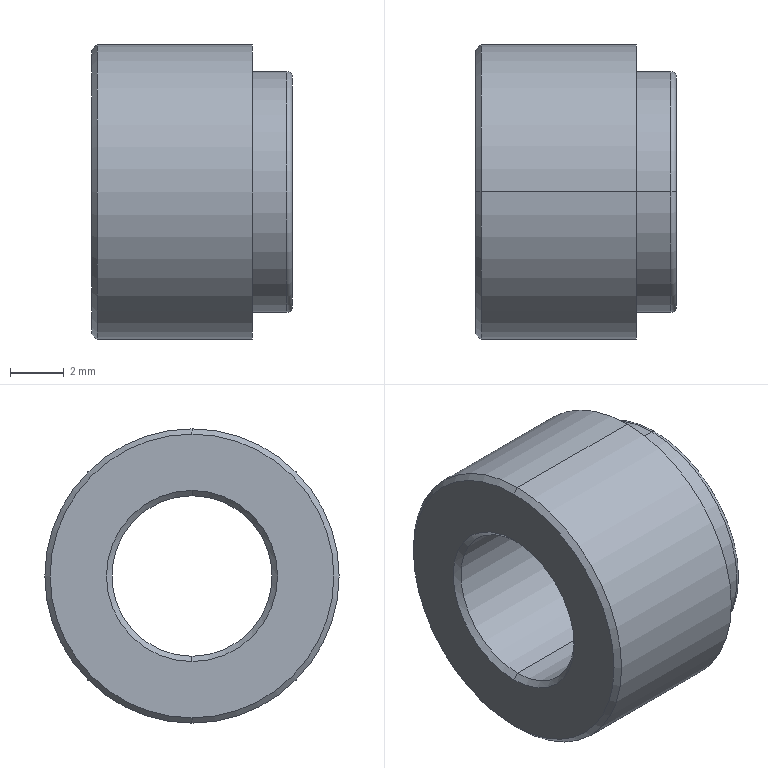Part | SolidWorks | features Chamfer 1, Extrusion 1, Fillet 1, ICE 1 | 2 solids | 20 faces | box 7.5 x 11 x 11 mm | volume 452.095 mm3 | cylinder 8 | cone 4 | plane 4 | torus 4 | commonest cylinder face diameters 6 x4 9 x2 11 x2
STEP:
#1=CARTESIAN_POINT('',(0.,0.,5.3));
#2=VERTEX_POINT('',#1);
#3=CARTESIAN_POINT('',(0.,0.,-5.3));
#4=VERTEX_POINT('',#3);
#5=CARTESIAN_POINT('',(0.,0.,0.));
#6=DIRECTION('',(-1.,0.,0.));
#7=DIRECTION('',(0.,0.,-1.));
#8=AXIS2_PLACEMENT_3D('',#5,#6,#7);
#9=CIRCLE('',#8,5.3);
#10=EDGE_CURVE('',#2,#4,#9,.T.);
#11=ORIENTED_EDGE('',*,*,#10,.F.);
#12=CARTESIAN_POINT('',(0.2,0.,5.5));
#13=VERTEX_POINT('',#12);
#14=CARTESIAN_POINT('',(0.2,0.,5.5));
#15=DIRECTION('',(0.7071,0.,0.7071));
#16=VECTOR('',#15,1000.);
#17=LINE('',#14,#16);
#18=EDGE_CURVE('',#2,#13,#17,.T.);
#19=ORIENTED_EDGE('',*,*,#18,.T.);
#20=CARTESIAN_POINT('',(0.2,0.,-5.5));
#21=VERTEX_POINT('',#20);
#22=CARTESIAN_POINT('',(0.2,0.,0.));
#23=DIRECTION('',(1.,0.,0.));
#24=DIRECTION('',(0.,0.,-1.));
#25=AXIS2_PLACEMENT_3D('',#22,#23,#24);
#26=CIRCLE('',#25,5.5);
#27=EDGE_CURVE('',#21,#13,#26,.T.);
#28=ORIENTED_EDGE('',*,*,#27,.F.);
#29=CARTESIAN_POINT('',(0.2,0.,-5.5));
#30=DIRECTION('',(0.7071,0.,-0.7071));
#31=VECTOR('',#30,1000.);
#32=LINE('',#29,#31);
#33=EDGE_CURVE('',#4,#21,#32,.T.);
#34=ORIENTED_EDGE('',*,*,#33,.F.);
#35=EDGE_LOOP('',(#11,#19,#28,#34));
#36=FACE_OUTER_BOUND('',#35,.T.);
#37=CARTESIAN_POINT('',(0.2,0.,0.));
#38=DIRECTION('',(1.,0.,0.));
#39=DIRECTION('',(0.,0.,-1.));
#40=AXIS2_PLACEMENT_3D('',#37,#38,#39);
#41=CONICAL_SURFACE('',#40,5.5,0.7854);
#42=ADVANCED_FACE('',(#36),#41,.T.);
#43=CARTESIAN_POINT('',(0.2,0.,-3.));
#44=VERTEX_POINT('',#43);
#45=CARTESIAN_POINT('',(0.2,0.,3.));
#46=VERTEX_POINT('',#45);
#47=CARTESIAN_POINT('',(0.2,0.,0.));
#48=DIRECTION('',(-1.,0.,0.));
#49=DIRECTION('',(0.,0.,-1.));
#50=AXIS2_PLACEMENT_3D('',#47,#48,#49);
#51=CIRCLE('',#50,3.);
#52=EDGE_CURVE('',#44,#46,#51,.T.);
#53=ORIENTED_EDGE('',*,*,#52,.F.);
#54=CARTESIAN_POINT('',(0.,0.,-3.2));
#55=VERTEX_POINT('',#54);
#56=CARTESIAN_POINT('',(0.,0.,-3.2));
#57=DIRECTION('',(-0.7071,0.,-0.7071));
#58=VECTOR('',#57,1000.);
#59=LINE('',#56,#58);
#60=EDGE_CURVE('',#44,#55,#59,.T.);
#61=ORIENTED_EDGE('',*,*,#60,.T.);
#62=CARTESIAN_POINT('',(0.,0.,3.2));
#63=VERTEX_POINT('',#62);
#64=CARTESIAN_POINT('',(0.,0.,0.));
#65=DIRECTION('',(1.,0.,0.));
#66=DIRECTION('',(0.,0.,-1.));
#67=AXIS2_PLACEMENT_3D('',#64,#65,#66);
#68=CIRCLE('',#67,3.2);
#69=EDGE_CURVE('',#63,#55,#68,.T.);
#70=ORIENTED_EDGE('',*,*,#69,.F.);
#71=CARTESIAN_POINT('',(0.,0.,3.2));
#72=DIRECTION('',(-0.7071,0.,0.7071));
#73=VECTOR('',#72,1000.);
#74=LINE('',#71,#73);
#75=EDGE_CURVE('',#46,#63,#74,.T.);
#76=ORIENTED_EDGE('',*,*,#75,.F.);
#77=EDGE_LOOP('',(#53,#61,#70,#76));
#78=FACE_OUTER_BOUND('',#77,.T.);
#79=CARTESIAN_POINT('',(0.,0.,0.));
#80=DIRECTION('',(-1.,0.,0.));
#81=DIRECTION('',(0.,0.,1.));
#82=AXIS2_PLACEMENT_3D('',#79,#80,#81);
#83=CONICAL_SURFACE('',#82,3.2,0.7854);
#84=ADVANCED_FACE('',(#78),#83,.F.);
#85=CARTESIAN_POINT('',(6.,0.,3.));
#86=VERTEX_POINT('',#85);
#87=CARTESIAN_POINT('',(6.,0.,-3.));
#88=VERTEX_POINT('',#87);
#89=CARTESIAN_POINT('',(6.,0.,0.));
#90=DIRECTION('',(1.,0.,0.));
#91=DIRECTION('',(0.,0.,-1.));
#92=AXIS2_PLACEMENT_3D('',#89,#90,#91);
#93=CIRCLE('',#92,3.);
#94=EDGE_CURVE('',#86,#88,#93,.T.);
#95=ORIENTED_EDGE('',*,*,#94,.T.);
#96=CARTESIAN_POINT('',(6.,0.,-3.));
#97=DIRECTION('',(-1.,0.,0.));
#98=VECTOR('',#97,1000.);
#99=LINE('',#96,#98);
#100=EDGE_CURVE('',#88,#44,#99,.T.);
#101=ORIENTED_EDGE('',*,*,#100,.T.);
#102=ORIENTED_EDGE('',*,*,#52,.T.);
#103=CARTESIAN_POINT('',(6.,0.,3.));
#104=DIRECTION('',(-1.,0.,0.));
#105=VECTOR('',#104,1000.);
#106=LINE('',#103,#105);
#107=EDGE_CURVE('',#86,#46,#106,.T.);
#108=ORIENTED_EDGE('',*,*,#107,.F.);
#109=EDGE_LOOP('',(#95,#101,#102,#108));
#110=FACE_OUTER_BOUND('',#109,.T.);
#111=CARTESIAN_POINT('',(6.,0.,0.));
#112=DIRECTION('',(-1.,0.,0.));
#113=DIRECTION('',(0.,0.,1.));
#114=AXIS2_PLACEMENT_3D('',#111,#112,#113);
#115=CYLINDRICAL_SURFACE('',#114,3.);
#116=ADVANCED_FACE('',(#110),#115,.F.);
#117=CARTESIAN_POINT('',(6.,0.,-5.5));
#118=VERTEX_POINT('',#117);
#119=CARTESIAN_POINT('',(6.,0.,5.5));
#120=VERTEX_POINT('',#119);
#121=CARTESIAN_POINT('',(6.,0.,0.));
#122=DIRECTION('',(1.,0.,0.));
#123=DIRECTION('',(0.,0.,-1.));
#124=AXIS2_PLACEMENT_3D('',#121,#122,#123);
#125=CIRCLE('',#124,5.5);
#126=EDGE_CURVE('',#118,#120,#125,.T.);
#127=ORIENTED_EDGE('',*,*,#126,.F.);
#128=CARTESIAN_POINT('',(6.,0.,-5.5));
#129=DIRECTION('',(-1.,0.,0.));
#130=VECTOR('',#129,1000.);
#131=LINE('',#128,#130);
#132=EDGE_CURVE('',#118,#21,#131,.T.);
#133=ORIENTED_EDGE('',*,*,#132,.T.);
#134=ORIENTED_EDGE('',*,*,#27,.T.);
#135=CARTESIAN_POINT('',(6.,0.,5.5));
#136=DIRECTION('',(-1.,0.,0.));
#137=VECTOR('',#136,1000.);
#138=LINE('',#135,#137);
#139=EDGE_CURVE('',#120,#13,#138,.T.);
#140=ORIENTED_EDGE('',*,*,#139,.F.);
#141=EDGE_LOOP('',(#127,#133,#134,#140));
#142=FACE_OUTER_BOUND('',#141,.T.);
#143=CARTESIAN_POINT('',(6.,0.,0.));
#144=DIRECTION('',(-1.,0.,0.));
#145=DIRECTION('',(0.,0.,1.));
#146=AXIS2_PLACEMENT_3D('',#143,#144,#145);
#147=CYLINDRICAL_SURFACE('',#146,5.5);
#148=ADVANCED_FACE('',(#142),#147,.T.);
#149=CARTESIAN_POINT('',(6.,0.,0.));
#150=DIRECTION('',(1.,0.,0.));
#151=DIRECTION('',(0.,0.,-1.));
#152=AXIS2_PLACEMENT_3D('',#149,#150,#151);
#153=CIRCLE('',#152,5.5);
#154=EDGE_CURVE('',#120,#118,#153,.T.);
#155=ORIENTED_EDGE('',*,*,#154,.T.);
#156=ORIENTED_EDGE('',*,*,#126,.T.);
#157=EDGE_LOOP('',(#155,#156));
#158=FACE_OUTER_BOUND('',#157,.T.);
#159=ORIENTED_EDGE('',*,*,#94,.F.);
#160=CARTESIAN_POINT('',(6.,0.,0.));
#161=DIRECTION('',(1.,0.,0.));
#162=DIRECTION('',(0.,0.,-1.));
#163=AXIS2_PLACEMENT_3D('',#160,#161,#162);
#164=CIRCLE('',#163,3.);
#165=EDGE_CURVE('',#88,#86,#164,.T.);
#166=ORIENTED_EDGE('',*,*,#165,.F.);
#167=EDGE_LOOP('',(#159,#166));
#168=FACE_BOUND('',#167,.T.);
#169=CARTESIAN_POINT('',(6.,0.,0.));
#170=DIRECTION('',(1.,0.,0.));
#171=DIRECTION('',(0.,0.,-1.));
#172=AXIS2_PLACEMENT_3D('',#169,#170,#171);
#173=PLANE('',#172);
#174=ADVANCED_FACE('',(#158,#168),#173,.T.);
#175=ORIENTED_EDGE('',*,*,#69,.T.);
#176=CARTESIAN_POINT('',(0.,0.,0.));
#177=DIRECTION('',(1.,0.,0.));
#178=DIRECTION('',(0.,0.,-1.));
#179=AXIS2_PLACEMENT_3D('',#176,#177,#178);
#180=CIRCLE('',#179,3.2);
#181=EDGE_CURVE('',#55,#63,#180,.T.);
#182=ORIENTED_EDGE('',*,*,#181,.T.);
#183=EDGE_LOOP('',(#175,#182));
#184=FACE_BOUND('',#183,.T.);
#185=CARTESIAN_POINT('',(0.,0.,0.));
#186=DIRECTION('',(-1.,0.,0.));
#187=DIRECTION('',(0.,0.,-1.));
#188=AXIS2_PLACEMENT_3D('',#185,#186,#187);
#189=CIRCLE('',#188,5.3);
#190=EDGE_CURVE('',#4,#2,#189,.T.);
#191=ORIENTED_EDGE('',*,*,#190,.T.);
#192=ORIENTED_EDGE('',*,*,#10,.T.);
#193=EDGE_LOOP('',(#191,#192));
#194=FACE_OUTER_BOUND('',#193,.T.);
#195=CARTESIAN_POINT('',(0.,0.,0.));
#196=DIRECTION('',(1.,0.,0.));
#197=DIRECTION('',(0.,0.,-1.));
#198=AXIS2_PLACEMENT_3D('',#195,#196,#197);
#199=PLANE('',#198);
#200=ADVANCED_FACE('',(#184,#194),#199,.F.);
#201=ORIENTED_EDGE('',*,*,#132,.F.);
#202=ORIENTED_EDGE('',*,*,#154,.F.);
#203=ORIENTED_EDGE('',*,*,#139,.T.);
#204=CARTESIAN_POINT('',(0.2,0.,0.));
#205=DIRECTION('',(1.,0.,0.));
#206=DIRECTION('',(0.,0.,-1.));
#207=AXIS2_PLACEMENT_3D('',#204,#205,#206);
#208=CIRCLE('',#207,5.5);
#209=EDGE_CURVE('',#13,#21,#208,.T.);
#210=ORIENTED_EDGE('',*,*,#209,.T.);
#211=EDGE_LOOP('',(#201,#202,#203,#210));
#212=FACE_OUTER_BOUND('',#211,.T.);
#213=CARTESIAN_POINT('',(6.,0.,0.));
#214=DIRECTION('',(-1.,0.,0.));
#215=DIRECTION('',(0.,0.,1.));
#216=AXIS2_PLACEMENT_3D('',#213,#214,#215);
#217=CYLINDRICAL_SURFACE('',#216,5.5);
#218=ADVANCED_FACE('',(#212),#217,.T.);
#219=ORIENTED_EDGE('',*,*,#100,.F.);
#220=ORIENTED_EDGE('',*,*,#165,.T.);
#221=ORIENTED_EDGE('',*,*,#107,.T.);
#222=CARTESIAN_POINT('',(0.2,0.,0.));
#223=DIRECTION('',(-1.,0.,0.));
#224=DIRECTION('',(0.,0.,-1.));
#225=AXIS2_PLACEMENT_3D('',#222,#223,#224);
#226=CIRCLE('',#225,3.);
#227=EDGE_CURVE('',#46,#44,#226,.T.);
#228=ORIENTED_EDGE('',*,*,#227,.T.);
#229=EDGE_LOOP('',(#219,#220,#221,#228));
#230=FACE_OUTER_BOUND('',#229,.T.);
#231=CARTESIAN_POINT('',(6.,0.,0.));
#232=DIRECTION('',(-1.,0.,0.));
#233=DIRECTION('',(0.,0.,1.));
#234=AXIS2_PLACEMENT_3D('',#231,#232,#233);
#235=CYLINDRICAL_SURFACE('',#234,3.);
#236=ADVANCED_FACE('',(#230),#235,.F.);
#237=ORIENTED_EDGE('',*,*,#60,.F.);
#238=ORIENTED_EDGE('',*,*,#227,.F.);
#239=ORIENTED_EDGE('',*,*,#75,.T.);
#240=ORIENTED_EDGE('',*,*,#181,.F.);
#241=EDGE_LOOP('',(#237,#238,#239,#240));
#242=FACE_OUTER_BOUND('',#241,.T.);
#243=CARTESIAN_POINT('',(0.,0.,0.));
#244=DIRECTION('',(-1.,0.,0.));
#245=DIRECTION('',(0.,0.,1.));
#246=AXIS2_PLACEMENT_3D('',#243,#244,#245);
#247=CONICAL_SURFACE('',#246,3.2,0.7854);
#248=ADVANCED_FACE('',(#242),#247,.F.);
#249=ORIENTED_EDGE('',*,*,#18,.F.);
#250=ORIENTED_EDGE('',*,*,#190,.F.);
#251=ORIENTED_EDGE('',*,*,#33,.T.);
#252=ORIENTED_EDGE('',*,*,#209,.F.);
#253=EDGE_LOOP('',(#249,#250,#251,#252));
#254=FACE_OUTER_BOUND('',#253,.T.);
#255=CARTESIAN_POINT('',(0.2,0.,0.));
#256=DIRECTION('',(1.,0.,0.));
#257=DIRECTION('',(0.,0.,-1.));
#258=AXIS2_PLACEMENT_3D('',#255,#256,#257);
#259=CONICAL_SURFACE('',#258,5.5,0.7854);
#260=ADVANCED_FACE('',(#254),#259,.T.);
#261=CLOSED_SHELL('',(#42,#84,#116,#148,#174,#200,#218,#236,#248,#260));
#262=MANIFOLD_SOLID_BREP('',#261);
#263=CARTESIAN_POINT('',(7.5,0.,3.2));
#264=VERTEX_POINT('',#263);
#265=CARTESIAN_POINT('',(7.5,0.,-3.2));
#266=VERTEX_POINT('',#265);
#267=CARTESIAN_POINT('',(7.5,0.,0.));
#268=DIRECTION('',(-1.,0.,0.));
#269=DIRECTION('',(0.,0.,-1.));
#270=AXIS2_PLACEMENT_3D('',#267,#268,#269);
#271=CIRCLE('',#270,3.2);
#272=EDGE_CURVE('',#264,#266,#271,.T.);
#273=ORIENTED_EDGE('',*,*,#272,.F.);
#274=CARTESIAN_POINT('',(7.3,0.,3.));
#275=VERTEX_POINT('',#274);
#276=CARTESIAN_POINT('',(7.3,0.,3.2));
#277=DIRECTION('',(0.,1.,0.));
#278=DIRECTION('',(0.,0.,1.));
#279=AXIS2_PLACEMENT_3D('',#276,#277,#278);
#280=CIRCLE('',#279,0.2);
#281=EDGE_CURVE('',#264,#275,#280,.T.);
#282=ORIENTED_EDGE('',*,*,#281,.T.);
#283=CARTESIAN_POINT('',(7.3,0.,-3.));
#284=VERTEX_POINT('',#283);
#285=CARTESIAN_POINT('',(7.3,0.,0.));
#286=DIRECTION('',(1.,0.,0.));
#287=DIRECTION('',(0.,0.,-1.));
#288=AXIS2_PLACEMENT_3D('',#285,#286,#287);
#289=CIRCLE('',#288,3.);
#290=EDGE_CURVE('',#284,#275,#289,.T.);
#291=ORIENTED_EDGE('',*,*,#290,.F.);
#292=CARTESIAN_POINT('',(7.3,0.,-3.2));
#293=DIRECTION('',(0.,-1.,0.));
#294=DIRECTION('',(0.,0.,-1.));
#295=AXIS2_PLACEMENT_3D('',#292,#293,#294);
#296=CIRCLE('',#295,0.2);
#297=EDGE_CURVE('',#266,#284,#296,.T.);
#298=ORIENTED_EDGE('',*,*,#297,.F.);
#299=EDGE_LOOP('',(#273,#282,#291,#298));
#300=FACE_OUTER_BOUND('',#299,.T.);
#301=CARTESIAN_POINT('',(7.3,0.,0.));
#302=DIRECTION('',(1.,0.,0.));
#303=DIRECTION('',(0.,0.,-1.));
#304=AXIS2_PLACEMENT_3D('',#301,#302,#303);
#305=TOROIDAL_SURFACE('',#304,3.2,0.2);
#306=ADVANCED_FACE('',(#300),#305,.T.);
#307=CARTESIAN_POINT('',(7.3,0.,4.5));
#308=VERTEX_POINT('',#307);
#309=CARTESIAN_POINT('',(7.3,0.,-4.5));
#310=VERTEX_POINT('',#309);
#311=CARTESIAN_POINT('',(7.3,0.,0.));
#312=DIRECTION('',(-1.,0.,0.));
#313=DIRECTION('',(0.,0.,-1.));
#314=AXIS2_PLACEMENT_3D('',#311,#312,#313);
#315=CIRCLE('',#314,4.5);
#316=EDGE_CURVE('',#308,#310,#315,.T.);
#317=ORIENTED_EDGE('',*,*,#316,.F.);
#318=CARTESIAN_POINT('',(7.5,0.,4.3));
#319=VERTEX_POINT('',#318);
#320=CARTESIAN_POINT('',(7.3,0.,4.3));
#321=DIRECTION('',(0.,1.,0.));
#322=DIRECTION('',(0.,0.,1.));
#323=AXIS2_PLACEMENT_3D('',#320,#321,#322);
#324=CIRCLE('',#323,0.2);
#325=EDGE_CURVE('',#308,#319,#324,.T.);
#326=ORIENTED_EDGE('',*,*,#325,.T.);
#327=CARTESIAN_POINT('',(7.5,0.,-4.3));
#328=VERTEX_POINT('',#327);
#329=CARTESIAN_POINT('',(7.5,0.,0.));
#330=DIRECTION('',(1.,0.,0.));
#331=DIRECTION('',(0.,0.,-1.));
#332=AXIS2_PLACEMENT_3D('',#329,#330,#331);
#333=CIRCLE('',#332,4.3);
#334=EDGE_CURVE('',#328,#319,#333,.T.);
#335=ORIENTED_EDGE('',*,*,#334,.F.);
#336=CARTESIAN_POINT('',(7.3,0.,-4.3));
#337=DIRECTION('',(0.,-1.,0.));
#338=DIRECTION('',(0.,0.,-1.));
#339=AXIS2_PLACEMENT_3D('',#336,#337,#338);
#340=CIRCLE('',#339,0.2);
#341=EDGE_CURVE('',#310,#328,#340,.T.);
#342=ORIENTED_EDGE('',*,*,#341,.F.);
#343=EDGE_LOOP('',(#317,#326,#335,#342));
#344=FACE_OUTER_BOUND('',#343,.T.);
#345=CARTESIAN_POINT('',(7.3,0.,0.));
#346=DIRECTION('',(1.,0.,0.));
#347=DIRECTION('',(0.,0.,-1.));
#348=AXIS2_PLACEMENT_3D('',#345,#346,#347);
#349=TOROIDAL_SURFACE('',#348,4.3,0.2);
#350=ADVANCED_FACE('',(#344),#349,.T.);
#351=CARTESIAN_POINT('',(7.3,0.,0.));
#352=DIRECTION('',(1.,0.,0.));
#353=DIRECTION('',(0.,0.,-1.));
#354=AXIS2_PLACEMENT_3D('',#351,#352,#353);
#355=CIRCLE('',#354,3.);
#356=EDGE_CURVE('',#275,#284,#355,.T.);
#357=ORIENTED_EDGE('',*,*,#356,.T.);
#358=CARTESIAN_POINT('',(6.,0.,-3.));
#359=VERTEX_POINT('',#358);
#360=CARTESIAN_POINT('',(7.5,0.,-3.));
#361=DIRECTION('',(-1.,0.,0.));
#362=VECTOR('',#361,1000.);
#363=LINE('',#360,#362);
#364=EDGE_CURVE('',#284,#359,#363,.T.);
#365=ORIENTED_EDGE('',*,*,#364,.T.);
#366=CARTESIAN_POINT('',(6.,0.,3.));
#367=VERTEX_POINT('',#366);
#368=CARTESIAN_POINT('',(6.,0.,0.));
#369=DIRECTION('',(1.,0.,0.));
#370=DIRECTION('',(0.,0.,-1.));
#371=AXIS2_PLACEMENT_3D('',#368,#369,#370);
#372=CIRCLE('',#371,3.);
#373=EDGE_CURVE('',#367,#359,#372,.T.);
#374=ORIENTED_EDGE('',*,*,#373,.F.);
#375=CARTESIAN_POINT('',(7.5,0.,3.));
#376=DIRECTION('',(-1.,0.,0.));
#377=VECTOR('',#376,1000.);
#378=LINE('',#375,#377);
#379=EDGE_CURVE('',#275,#367,#378,.T.);
#380=ORIENTED_EDGE('',*,*,#379,.F.);
#381=EDGE_LOOP('',(#357,#365,#374,#380));
#382=FACE_OUTER_BOUND('',#381,.T.);
#383=CARTESIAN_POINT('',(7.5,0.,0.));
#384=DIRECTION('',(-1.,0.,0.));
#385=DIRECTION('',(0.,0.,1.));
#386=AXIS2_PLACEMENT_3D('',#383,#384,#385);
#387=CYLINDRICAL_SURFACE('',#386,3.);
#388=ADVANCED_FACE('',(#382),#387,.F.);
#389=ORIENTED_EDGE('',*,*,#316,.T.);
#390=CARTESIAN_POINT('',(6.,0.,-4.5));
#391=VERTEX_POINT('',#390);
#392=CARTESIAN_POINT('',(7.5,0.,-4.5));
#393=DIRECTION('',(-1.,0.,0.));
#394=VECTOR('',#393,1000.);
#395=LINE('',#392,#394);
#396=EDGE_CURVE('',#310,#391,#395,.T.);
#397=ORIENTED_EDGE('',*,*,#396,.T.);
#398=CARTESIAN_POINT('',(6.,0.,4.5));
#399=VERTEX_POINT('',#398);
#400=CARTESIAN_POINT('',(6.,0.,0.));
#401=DIRECTION('',(1.,0.,0.));
#402=DIRECTION('',(0.,0.,-1.));
#403=AXIS2_PLACEMENT_3D('',#400,#401,#402);
#404=CIRCLE('',#403,4.5);
#405=EDGE_CURVE('',#391,#399,#404,.T.);
#406=ORIENTED_EDGE('',*,*,#405,.T.);
#407=CARTESIAN_POINT('',(7.5,0.,4.5));
#408=DIRECTION('',(-1.,0.,0.));
#409=VECTOR('',#408,1000.);
#410=LINE('',#407,#409);
#411=EDGE_CURVE('',#308,#399,#410,.T.);
#412=ORIENTED_EDGE('',*,*,#411,.F.);
#413=EDGE_LOOP('',(#389,#397,#406,#412));
#414=FACE_OUTER_BOUND('',#413,.T.);
#415=CARTESIAN_POINT('',(7.5,0.,0.));
#416=DIRECTION('',(-1.,0.,0.));
#417=DIRECTION('',(0.,0.,1.));
#418=AXIS2_PLACEMENT_3D('',#415,#416,#417);
#419=CYLINDRICAL_SURFACE('',#418,4.5);
#420=ADVANCED_FACE('',(#414),#419,.T.);
#421=ORIENTED_EDGE('',*,*,#334,.T.);
#422=CARTESIAN_POINT('',(7.5,0.,0.));
#423=DIRECTION('',(1.,0.,0.));
#424=DIRECTION('',(0.,0.,-1.));
#425=AXIS2_PLACEMENT_3D('',#422,#423,#424);
#426=CIRCLE('',#425,4.3);
#427=EDGE_CURVE('',#319,#328,#426,.T.);
#428=ORIENTED_EDGE('',*,*,#427,.T.);
#429=EDGE_LOOP('',(#421,#428));
#430=FACE_OUTER_BOUND('',#429,.T.);
#431=CARTESIAN_POINT('',(7.5,0.,0.));
#432=DIRECTION('',(-1.,0.,0.));
#433=DIRECTION('',(0.,0.,-1.));
#434=AXIS2_PLACEMENT_3D('',#431,#432,#433);
#435=CIRCLE('',#434,3.2);
#436=EDGE_CURVE('',#266,#264,#435,.T.);
#437=ORIENTED_EDGE('',*,*,#436,.T.);
#438=ORIENTED_EDGE('',*,*,#272,.T.);
#439=EDGE_LOOP('',(#437,#438));
#440=FACE_BOUND('',#439,.T.);
#441=CARTESIAN_POINT('',(7.5,0.,0.));
#442=DIRECTION('',(1.,0.,0.));
#443=DIRECTION('',(0.,0.,-1.));
#444=AXIS2_PLACEMENT_3D('',#441,#442,#443);
#445=PLANE('',#444);
#446=ADVANCED_FACE('',(#430,#440),#445,.T.);
#447=CARTESIAN_POINT('',(6.,0.,0.));
#448=DIRECTION('',(1.,0.,0.));
#449=DIRECTION('',(0.,0.,-1.));
#450=AXIS2_PLACEMENT_3D('',#447,#448,#449);
#451=CIRCLE('',#450,4.5);
#452=EDGE_CURVE('',#399,#391,#451,.T.);
#453=ORIENTED_EDGE('',*,*,#452,.F.);
#454=ORIENTED_EDGE('',*,*,#405,.F.);
#455=EDGE_LOOP('',(#453,#454));
#456=FACE_OUTER_BOUND('',#455,.T.);
#457=ORIENTED_EDGE('',*,*,#373,.T.);
#458=CARTESIAN_POINT('',(6.,0.,0.));
#459=DIRECTION('',(1.,0.,0.));
#460=DIRECTION('',(0.,0.,-1.));
#461=AXIS2_PLACEMENT_3D('',#458,#459,#460);
#462=CIRCLE('',#461,3.);
#463=EDGE_CURVE('',#359,#367,#462,.T.);
#464=ORIENTED_EDGE('',*,*,#463,.T.);
#465=EDGE_LOOP('',(#457,#464));
#466=FACE_BOUND('',#465,.T.);
#467=CARTESIAN_POINT('',(6.,0.,0.));
#468=DIRECTION('',(1.,0.,0.));
#469=DIRECTION('',(0.,0.,-1.));
#470=AXIS2_PLACEMENT_3D('',#467,#468,#469);
#471=PLANE('',#470);
#472=ADVANCED_FACE('',(#456,#466),#471,.F.);
#473=ORIENTED_EDGE('',*,*,#396,.F.);
#474=CARTESIAN_POINT('',(7.3,0.,0.));
#475=DIRECTION('',(-1.,0.,0.));
#476=DIRECTION('',(0.,0.,-1.));
#477=AXIS2_PLACEMENT_3D('',#474,#475,#476);
#478=CIRCLE('',#477,4.5);
#479=EDGE_CURVE('',#310,#308,#478,.T.);
#480=ORIENTED_EDGE('',*,*,#479,.T.);
#481=ORIENTED_EDGE('',*,*,#411,.T.);
#482=ORIENTED_EDGE('',*,*,#452,.T.);
#483=EDGE_LOOP('',(#473,#480,#481,#482));
#484=FACE_OUTER_BOUND('',#483,.T.);
#485=CARTESIAN_POINT('',(7.5,0.,0.));
#486=DIRECTION('',(-1.,0.,0.));
#487=DIRECTION('',(0.,0.,1.));
#488=AXIS2_PLACEMENT_3D('',#485,#486,#487);
#489=CYLINDRICAL_SURFACE('',#488,4.5);
#490=ADVANCED_FACE('',(#484),#489,.T.);
#491=ORIENTED_EDGE('',*,*,#364,.F.);
#492=ORIENTED_EDGE('',*,*,#290,.T.);
#493=ORIENTED_EDGE('',*,*,#379,.T.);
#494=ORIENTED_EDGE('',*,*,#463,.F.);
#495=EDGE_LOOP('',(#491,#492,#493,#494));
#496=FACE_OUTER_BOUND('',#495,.T.);
#497=CARTESIAN_POINT('',(7.5,0.,0.));
#498=DIRECTION('',(-1.,0.,0.));
#499=DIRECTION('',(0.,0.,1.));
#500=AXIS2_PLACEMENT_3D('',#497,#498,#499);
#501=CYLINDRICAL_SURFACE('',#500,3.);
#502=ADVANCED_FACE('',(#496),#501,.F.);
#503=ORIENTED_EDGE('',*,*,#325,.F.);
#504=ORIENTED_EDGE('',*,*,#479,.F.);
#505=ORIENTED_EDGE('',*,*,#341,.T.);
#506=ORIENTED_EDGE('',*,*,#427,.F.);
#507=EDGE_LOOP('',(#503,#504,#505,#506));
#508=FACE_OUTER_BOUND('',#507,.T.);
#509=CARTESIAN_POINT('',(7.3,0.,0.));
#510=DIRECTION('',(1.,0.,0.));
#511=DIRECTION('',(0.,0.,-1.));
#512=AXIS2_PLACEMENT_3D('',#509,#510,#511);
#513=TOROIDAL_SURFACE('',#512,4.3,0.2);
#514=ADVANCED_FACE('',(#508),#513,.T.);
#515=ORIENTED_EDGE('',*,*,#281,.F.);
#516=ORIENTED_EDGE('',*,*,#436,.F.);
#517=ORIENTED_EDGE('',*,*,#297,.T.);
#518=ORIENTED_EDGE('',*,*,#356,.F.);
#519=EDGE_LOOP('',(#515,#516,#517,#518));
#520=FACE_OUTER_BOUND('',#519,.T.);
#521=CARTESIAN_POINT('',(7.3,0.,0.));
#522=DIRECTION('',(1.,0.,0.));
#523=DIRECTION('',(0.,0.,-1.));
#524=AXIS2_PLACEMENT_3D('',#521,#522,#523);
#525=TOROIDAL_SURFACE('',#524,3.2,0.2);
#526=ADVANCED_FACE('',(#520),#525,.T.);
#527=CLOSED_SHELL('',(#306,#350,#388,#420,#446,#472,#490,#502,#514,#526));
#528=MANIFOLD_SOLID_BREP('',#527);
#529=CARTESIAN_POINT('',(0.,0.,0.));
#530=DIRECTION('',(0.,0.,1.));
#531=DIRECTION('',(1.,0.,0.));
#532=AXIS2_PLACEMENT_3D('',#529,#530,#531);
#533=(LENGTH_UNIT()NAMED_UNIT(*)SI_UNIT(.MILLI.,.METRE.));
#534=UNCERTAINTY_MEASURE_WITH_UNIT(LENGTH_MEASURE(0.00001),#533,'','');
#535=(NAMED_UNIT(*)PLANE_ANGLE_UNIT()SI_UNIT($,.RADIAN.));
#536=(NAMED_UNIT(*)SI_UNIT($,.STERADIAN.)SOLID_ANGLE_UNIT());
#537=(GEOMETRIC_REPRESENTATION_CONTEXT(3)GLOBAL_UNCERTAINTY_ASSIGNED_CONTEXT((#534))GLOBAL_UNIT_ASSIGNED_CONTEXT((#533,#535,#536))REPRESENTATION_CONTEXT('',''));
#538=ADVANCED_BREP_SHAPE_REPRESENTATION('',(#262,#528,#532),#537);